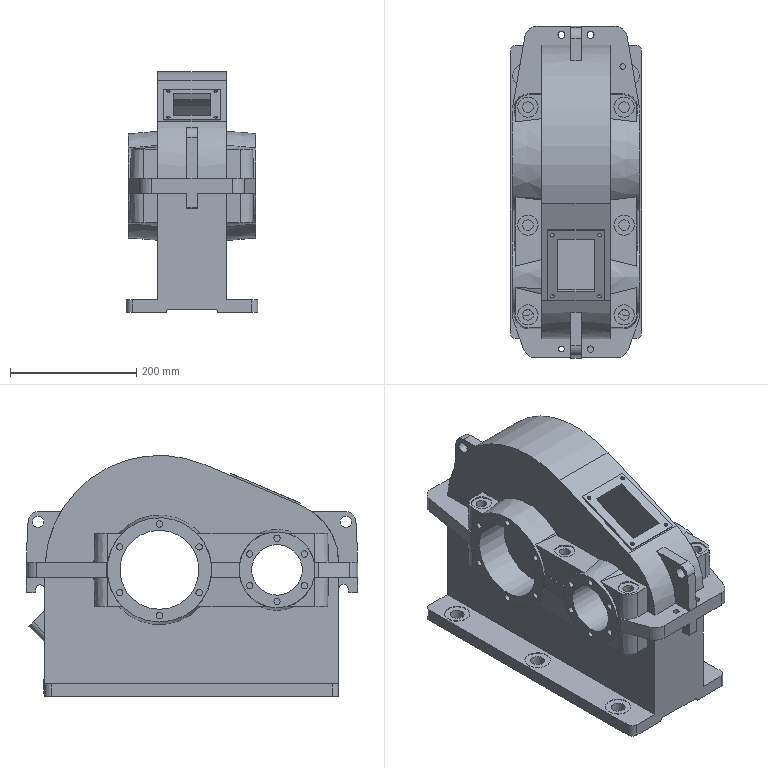Part | NX | features SIMPLE HOLE 56, DATUM_CSYS 26, HOLE PACKAGE 26, SKETCH 25, EXTRUDE 17, EXTRACT_FACE 16, EXTRACT_DATUM_AXIS 10, BLEND 8, CBORE_HOLE 7, EXTRACT_DATUM_PLANE 6, FSET 6, Instance Feature 5, Mirror Feature 5, DRAFT 4, EXTRACT_STRING 2 | 1 solid | 266 faces | box 208 x 525 x 381.222 mm | volume 7183001 mm3 | plane 156 | cylinder 96 | cone 14 | commonest cylinder face diameters 10 x28 32 x14 40 x10 17 x6 22 x6 4 x4